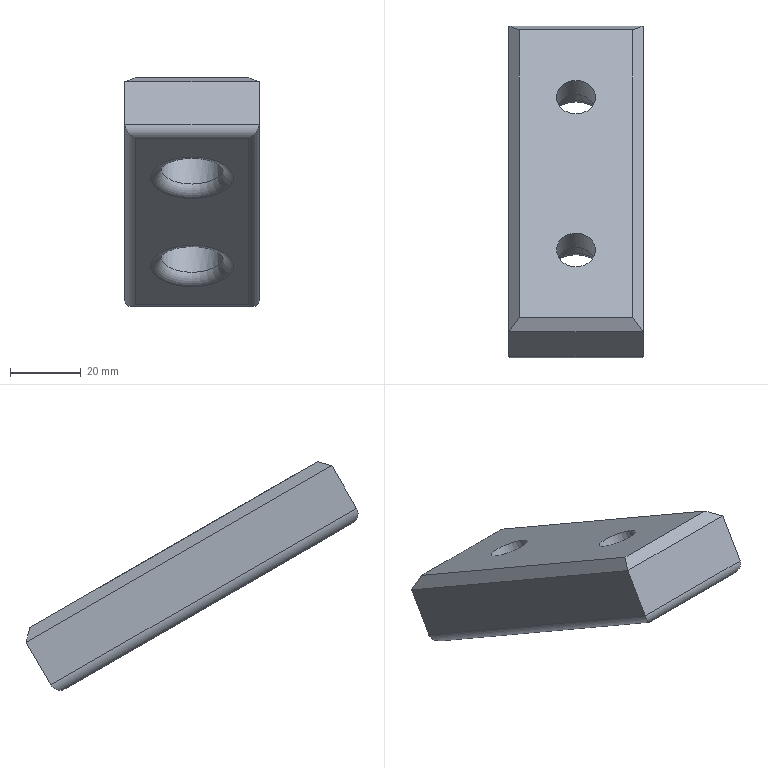Part | NX | features MAIN_BODY 2 | 1 solid | 22 faces | box 38 x 94.004 x 64.722 mm | volume 66749 mm3 | plane 12 | cylinder 8 | torus 2 | commonest cylinder face diameters 6 x4 11 x2 17.5 x2
STEP:
#1=CARTESIAN_POINT('',(222.,386.847,-246.44));
#2=VERTEX_POINT('',#1);
#3=CARTESIAN_POINT('',(222.,468.253,-293.44));
#4=VERTEX_POINT('',#3);
#5=CARTESIAN_POINT('',(222.,514.153,-319.94));
#6=DIRECTION('',(0.,-0.866,0.5));
#7=VECTOR('',#6,1000.);
#8=LINE('',#5,#7);
#9=EDGE_CURVE('',#2,#4,#8,.F.);
#10=ORIENTED_EDGE('',*,*,#9,.F.);
#11=CARTESIAN_POINT('',(190.,386.847,-246.44));
#12=VERTEX_POINT('',#11);
#13=CARTESIAN_POINT('',(225.,386.847,-246.44));
#14=DIRECTION('',(-1.,0.,0.));
#15=VECTOR('',#14,1000.);
#16=LINE('',#13,#15);
#17=EDGE_CURVE('',#12,#2,#16,.F.);
#18=ORIENTED_EDGE('',*,*,#17,.F.);
#19=CARTESIAN_POINT('',(190.,468.253,-293.44));
#20=VERTEX_POINT('',#19);
#21=CARTESIAN_POINT('',(190.,514.153,-319.94));
#22=DIRECTION('',(0.,0.866,-0.5));
#23=VECTOR('',#22,1000.);
#24=LINE('',#21,#23);
#25=EDGE_CURVE('',#20,#12,#24,.F.);
#26=ORIENTED_EDGE('',*,*,#25,.F.);
#27=CARTESIAN_POINT('',(225.,468.253,-293.44));
#28=DIRECTION('',(1.,0.,0.));
#29=VECTOR('',#28,1000.);
#30=LINE('',#27,#29);
#31=EDGE_CURVE('',#4,#20,#30,.F.);
#32=ORIENTED_EDGE('',*,*,#31,.F.);
#33=EDGE_LOOP('',(#10,#18,#26,#32));
#34=FACE_BOUND('',#33,.T.);
#35=CARTESIAN_POINT('',(206.,459.376,-288.315));
#36=VERTEX_POINT('',#35);
#37=CARTESIAN_POINT('',(206.,449.201,-282.44));
#38=DIRECTION('',(0.,0.5,0.866));
#39=DIRECTION('',(0.,0.866,-0.5));
#40=AXIS2_PLACEMENT_3D('',#37,#38,#39);
#41=CIRCLE('',#40,11.75);
#42=EDGE_CURVE('',#36,#36,#41,.F.);
#43=ORIENTED_EDGE('',*,*,#42,.F.);
#44=EDGE_LOOP('',(#43));
#45=FACE_BOUND('',#44,.T.);
#46=CARTESIAN_POINT('',(206.,416.075,-263.315));
#47=VERTEX_POINT('',#46);
#48=CARTESIAN_POINT('',(206.,405.899,-257.44));
#49=DIRECTION('',(0.,0.5,0.866));
#50=DIRECTION('',(0.,0.866,-0.5));
#51=AXIS2_PLACEMENT_3D('',#48,#49,#50);
#52=CIRCLE('',#51,11.75);
#53=EDGE_CURVE('',#47,#47,#52,.F.);
#54=ORIENTED_EDGE('',*,*,#53,.F.);
#55=EDGE_LOOP('',(#54));
#56=FACE_BOUND('',#55,.T.);
#57=CARTESIAN_POINT('',(225.,514.153,-319.94));
#58=DIRECTION('',(0.,-0.5,-0.866));
#59=DIRECTION('',(0.,0.866,-0.5));
#60=AXIS2_PLACEMENT_3D('',#57,#58,#59);
#61=PLANE('',#60);
#62=ADVANCED_FACE('',(#34,#45,#56),#61,.T.);
#63=CARTESIAN_POINT('',(200.5,459.201,-265.12));
#64=VERTEX_POINT('',#63);
#65=CARTESIAN_POINT('',(206.,459.201,-265.12));
#66=DIRECTION('',(0.,0.5,0.866));
#67=DIRECTION('',(-1.,0.,0.));
#68=AXIS2_PLACEMENT_3D('',#65,#66,#67);
#69=CIRCLE('',#68,5.5);
#70=EDGE_CURVE('',#64,#64,#69,.T.);
#71=ORIENTED_EDGE('',*,*,#70,.T.);
#72=EDGE_LOOP('',(#71));
#73=FACE_BOUND('',#72,.T.);
#74=CARTESIAN_POINT('',(206.,459.964,-274.798));
#75=VERTEX_POINT('',#74);
#76=CARTESIAN_POINT('',(206.,455.201,-272.048));
#77=DIRECTION('',(0.,0.5,0.866));
#78=DIRECTION('',(0.,0.866,-0.5));
#79=AXIS2_PLACEMENT_3D('',#76,#77,#78);
#80=CIRCLE('',#79,5.5);
#81=EDGE_CURVE('',#75,#75,#80,.T.);
#82=ORIENTED_EDGE('',*,*,#81,.F.);
#83=EDGE_LOOP('',(#82));
#84=FACE_BOUND('',#83,.T.);
#85=CARTESIAN_POINT('',(206.,449.201,-282.44));
#86=DIRECTION('',(0.,0.5,0.866));
#87=DIRECTION('',(0.,-0.866,0.5));
#88=AXIS2_PLACEMENT_3D('',#85,#86,#87);
#89=CYLINDRICAL_SURFACE('',#88,5.5);
#90=ADVANCED_FACE('',(#73,#84),#89,.F.);
#91=CARTESIAN_POINT('',(190.,396.847,-229.12));
#92=VERTEX_POINT('',#91);
#93=CARTESIAN_POINT('',(190.,478.253,-276.12));
#94=VERTEX_POINT('',#93);
#95=CARTESIAN_POINT('',(190.,524.153,-302.62));
#96=DIRECTION('',(0.,0.866,-0.5));
#97=VECTOR('',#96,1000.);
#98=LINE('',#95,#97);
#99=EDGE_CURVE('',#92,#94,#98,.T.);
#100=ORIENTED_EDGE('',*,*,#99,.F.);
#101=CARTESIAN_POINT('',(222.,396.847,-229.12));
#102=VERTEX_POINT('',#101);
#103=CARTESIAN_POINT('',(187.,396.847,-229.12));
#104=DIRECTION('',(-1.,0.,0.));
#105=VECTOR('',#104,1000.);
#106=LINE('',#103,#105);
#107=EDGE_CURVE('',#102,#92,#106,.T.);
#108=ORIENTED_EDGE('',*,*,#107,.F.);
#109=CARTESIAN_POINT('',(222.,478.253,-276.12));
#110=VERTEX_POINT('',#109);
#111=CARTESIAN_POINT('',(222.,394.249,-227.62));
#112=DIRECTION('',(0.,-0.866,0.5));
#113=VECTOR('',#112,1000.);
#114=LINE('',#111,#113);
#115=EDGE_CURVE('',#110,#102,#114,.T.);
#116=ORIENTED_EDGE('',*,*,#115,.F.);
#117=CARTESIAN_POINT('',(225.,478.253,-276.12));
#118=DIRECTION('',(1.,0.,0.));
#119=VECTOR('',#118,1000.);
#120=LINE('',#117,#119);
#121=EDGE_CURVE('',#94,#110,#120,.T.);
#122=ORIENTED_EDGE('',*,*,#121,.F.);
#123=EDGE_LOOP('',(#100,#108,#116,#122));
#124=FACE_BOUND('',#123,.T.);
#125=CARTESIAN_POINT('',(200.5,415.899,-240.12));
#126=VERTEX_POINT('',#125);
#127=CARTESIAN_POINT('',(206.,415.899,-240.12));
#128=DIRECTION('',(0.,-0.5,-0.866));
#129=DIRECTION('',(-1.,0.,0.));
#130=AXIS2_PLACEMENT_3D('',#127,#128,#129);
#131=CIRCLE('',#130,5.5);
#132=EDGE_CURVE('',#126,#126,#131,.T.);
#133=ORIENTED_EDGE('',*,*,#132,.T.);
#134=EDGE_LOOP('',(#133));
#135=FACE_BOUND('',#134,.T.);
#136=ORIENTED_EDGE('',*,*,#70,.F.);
#137=EDGE_LOOP('',(#136));
#138=FACE_BOUND('',#137,.T.);
#139=CARTESIAN_POINT('',(225.,524.153,-302.62));
#140=DIRECTION('',(0.,-0.5,-0.866));
#141=DIRECTION('',(0.,0.866,-0.5));
#142=AXIS2_PLACEMENT_3D('',#139,#140,#141);
#143=PLANE('',#142);
#144=ADVANCED_FACE('',(#124,#135,#138),#143,.F.);
#145=CARTESIAN_POINT('',(225.,385.749,-242.342));
#146=VERTEX_POINT('',#145);
#147=CARTESIAN_POINT('',(225.,392.749,-230.218));
#148=VERTEX_POINT('',#147);
#149=CARTESIAN_POINT('',(225.,384.249,-244.94));
#150=DIRECTION('',(0.,0.5,0.866));
#151=VECTOR('',#150,1000.);
#152=LINE('',#149,#151);
#153=EDGE_CURVE('',#146,#148,#152,.T.);
#154=ORIENTED_EDGE('',*,*,#153,.F.);
#155=CARTESIAN_POINT('',(225.,472.351,-292.342));
#156=VERTEX_POINT('',#155);
#157=CARTESIAN_POINT('',(225.,515.653,-317.342));
#158=DIRECTION('',(0.,-0.866,0.5));
#159=VECTOR('',#158,1000.);
#160=LINE('',#157,#159);
#161=EDGE_CURVE('',#156,#146,#160,.T.);
#162=ORIENTED_EDGE('',*,*,#161,.F.);
#163=CARTESIAN_POINT('',(225.,479.351,-280.218));
#164=VERTEX_POINT('',#163);
#165=CARTESIAN_POINT('',(225.,470.851,-294.94));
#166=DIRECTION('',(0.,0.5,0.866));
#167=VECTOR('',#166,1000.);
#168=LINE('',#165,#167);
#169=EDGE_CURVE('',#156,#164,#168,.T.);
#170=ORIENTED_EDGE('',*,*,#169,.T.);
#171=CARTESIAN_POINT('',(225.,522.653,-305.218));
#172=DIRECTION('',(0.,0.866,-0.5));
#173=VECTOR('',#172,1000.);
#174=LINE('',#171,#173);
#175=EDGE_CURVE('',#148,#164,#174,.T.);
#176=ORIENTED_EDGE('',*,*,#175,.F.);
#177=EDGE_LOOP('',(#154,#162,#170,#176));
#178=FACE_BOUND('',#177,.T.);
#179=CARTESIAN_POINT('',(225.,514.153,-319.94));
#180=DIRECTION('',(1.,0.,0.));
#181=DIRECTION('',(0.,0.866,-0.5));
#182=AXIS2_PLACEMENT_3D('',#179,#180,#181);
#183=PLANE('',#182);
#184=ADVANCED_FACE('',(#178),#183,.T.);
#185=CARTESIAN_POINT('',(187.,385.749,-242.342));
#186=VERTEX_POINT('',#185);
#187=CARTESIAN_POINT('',(187.,392.749,-230.218));
#188=VERTEX_POINT('',#187);
#189=CARTESIAN_POINT('',(187.,384.249,-244.94));
#190=DIRECTION('',(0.,0.5,0.866));
#191=VECTOR('',#190,1000.);
#192=LINE('',#189,#191);
#193=EDGE_CURVE('',#186,#188,#192,.T.);
#194=ORIENTED_EDGE('',*,*,#193,.F.);
#195=CARTESIAN_POINT('',(225.,385.749,-242.342));
#196=DIRECTION('',(-1.,0.,0.));
#197=VECTOR('',#196,1000.);
#198=LINE('',#195,#197);
#199=EDGE_CURVE('',#146,#186,#198,.T.);
#200=ORIENTED_EDGE('',*,*,#199,.F.);
#201=ORIENTED_EDGE('',*,*,#153,.T.);
#202=CARTESIAN_POINT('',(225.,392.749,-230.218));
#203=DIRECTION('',(1.,0.,0.));
#204=VECTOR('',#203,1000.);
#205=LINE('',#202,#204);
#206=EDGE_CURVE('',#188,#148,#205,.T.);
#207=ORIENTED_EDGE('',*,*,#206,.F.);
#208=EDGE_LOOP('',(#194,#200,#201,#207));
#209=FACE_BOUND('',#208,.T.);
#210=CARTESIAN_POINT('',(225.,384.249,-244.94));
#211=DIRECTION('',(0.,-0.866,0.5));
#212=DIRECTION('',(0.,-0.5,-0.866));
#213=AXIS2_PLACEMENT_3D('',#210,#211,#212);
#214=PLANE('',#213);
#215=ADVANCED_FACE('',(#209),#214,.T.);
#216=CARTESIAN_POINT('',(187.,472.351,-292.342));
#217=VERTEX_POINT('',#216);
#218=CARTESIAN_POINT('',(187.,479.351,-280.218));
#219=VERTEX_POINT('',#218);
#220=CARTESIAN_POINT('',(187.,470.851,-294.94));
#221=DIRECTION('',(0.,0.5,0.866));
#222=VECTOR('',#221,1000.);
#223=LINE('',#220,#222);
#224=EDGE_CURVE('',#217,#219,#223,.T.);
#225=ORIENTED_EDGE('',*,*,#224,.F.);
#226=CARTESIAN_POINT('',(187.,385.749,-242.342));
#227=DIRECTION('',(0.,0.866,-0.5));
#228=VECTOR('',#227,1000.);
#229=LINE('',#226,#228);
#230=EDGE_CURVE('',#186,#217,#229,.T.);
#231=ORIENTED_EDGE('',*,*,#230,.F.);
#232=ORIENTED_EDGE('',*,*,#193,.T.);
#233=CARTESIAN_POINT('',(187.,392.749,-230.218));
#234=DIRECTION('',(0.,-0.866,0.5));
#235=VECTOR('',#234,1000.);
#236=LINE('',#233,#235);
#237=EDGE_CURVE('',#219,#188,#236,.T.);
#238=ORIENTED_EDGE('',*,*,#237,.F.);
#239=EDGE_LOOP('',(#225,#231,#232,#238));
#240=FACE_BOUND('',#239,.T.);
#241=CARTESIAN_POINT('',(187.,384.249,-244.94));
#242=DIRECTION('',(-1.,0.,0.));
#243=DIRECTION('',(0.,-0.866,0.5));
#244=AXIS2_PLACEMENT_3D('',#241,#242,#243);
#245=PLANE('',#244);
#246=ADVANCED_FACE('',(#240),#245,.T.);
#247=ORIENTED_EDGE('',*,*,#169,.F.);
#248=CARTESIAN_POINT('',(187.,472.351,-292.342));
#249=DIRECTION('',(1.,0.,0.));
#250=VECTOR('',#249,1000.);
#251=LINE('',#248,#250);
#252=EDGE_CURVE('',#217,#156,#251,.T.);
#253=ORIENTED_EDGE('',*,*,#252,.F.);
#254=ORIENTED_EDGE('',*,*,#224,.T.);
#255=CARTESIAN_POINT('',(187.,479.351,-280.218));
#256=DIRECTION('',(-1.,0.,0.));
#257=VECTOR('',#256,1000.);
#258=LINE('',#255,#257);
#259=EDGE_CURVE('',#164,#219,#258,.T.);
#260=ORIENTED_EDGE('',*,*,#259,.F.);
#261=EDGE_LOOP('',(#247,#253,#254,#260));
#262=FACE_BOUND('',#261,.T.);
#263=CARTESIAN_POINT('',(187.,470.851,-294.94));
#264=DIRECTION('',(0.,0.866,-0.5));
#265=DIRECTION('',(-1.,0.,0.));
#266=AXIS2_PLACEMENT_3D('',#263,#264,#265);
#267=PLANE('',#266);
#268=ADVANCED_FACE('',(#262),#267,.T.);
#269=CARTESIAN_POINT('',(206.,407.136,-244.298));
#270=VERTEX_POINT('',#269);
#271=CARTESIAN_POINT('',(206.,411.899,-247.048));
#272=DIRECTION('',(0.,-0.5,-0.866));
#273=DIRECTION('',(0.,-0.866,0.5));
#274=AXIS2_PLACEMENT_3D('',#271,#272,#273);
#275=CIRCLE('',#274,5.5);
#276=EDGE_CURVE('',#270,#270,#275,.F.);
#277=ORIENTED_EDGE('',*,*,#276,.F.);
#278=EDGE_LOOP('',(#277));
#279=FACE_BOUND('',#278,.T.);
#280=ORIENTED_EDGE('',*,*,#132,.F.);
#281=EDGE_LOOP('',(#280));
#282=FACE_BOUND('',#281,.T.);
#283=CARTESIAN_POINT('',(206.,405.899,-257.44));
#284=DIRECTION('',(0.,0.5,0.866));
#285=DIRECTION('',(0.,-0.866,0.5));
#286=AXIS2_PLACEMENT_3D('',#283,#284,#285);
#287=CYLINDRICAL_SURFACE('',#286,5.5);
#288=ADVANCED_FACE('',(#279,#282),#287,.F.);
#289=CARTESIAN_POINT('',(206.,458.278,-284.217));
#290=VERTEX_POINT('',#289);
#291=CARTESIAN_POINT('',(206.,450.701,-279.842));
#292=DIRECTION('',(0.,0.5,0.866));
#293=DIRECTION('',(0.,0.866,-0.5));
#294=AXIS2_PLACEMENT_3D('',#291,#292,#293);
#295=CIRCLE('',#294,8.75);
#296=EDGE_CURVE('',#290,#290,#295,.T.);
#297=ORIENTED_EDGE('',*,*,#296,.F.);
#298=EDGE_LOOP('',(#297));
#299=FACE_BOUND('',#298,.T.);
#300=CARTESIAN_POINT('',(197.25,455.201,-272.048));
#301=VERTEX_POINT('',#300);
#302=CARTESIAN_POINT('',(206.,455.201,-272.048));
#303=DIRECTION('',(0.,0.5,0.866));
#304=DIRECTION('',(-1.,0.,0.));
#305=AXIS2_PLACEMENT_3D('',#302,#303,#304);
#306=CIRCLE('',#305,8.75);
#307=EDGE_CURVE('',#301,#301,#306,.T.);
#308=ORIENTED_EDGE('',*,*,#307,.T.);
#309=EDGE_LOOP('',(#308));
#310=FACE_BOUND('',#309,.T.);
#311=CARTESIAN_POINT('',(206.,444.201,-291.1));
#312=DIRECTION('',(0.,0.5,0.866));
#313=DIRECTION('',(0.,-0.866,0.5));
#314=AXIS2_PLACEMENT_3D('',#311,#312,#313);
#315=CYLINDRICAL_SURFACE('',#314,8.75);
#316=ADVANCED_FACE('',(#299,#310),#315,.F.);
#317=ORIENTED_EDGE('',*,*,#81,.T.);
#318=EDGE_LOOP('',(#317));
#319=FACE_BOUND('',#318,.T.);
#320=ORIENTED_EDGE('',*,*,#307,.F.);
#321=EDGE_LOOP('',(#320));
#322=FACE_BOUND('',#321,.T.);
#323=CARTESIAN_POINT('',(206.,455.201,-272.048));
#324=DIRECTION('',(0.,-0.5,-0.866));
#325=DIRECTION('',(0.,0.866,-0.5));
#326=AXIS2_PLACEMENT_3D('',#323,#324,#325);
#327=PLANE('',#326);
#328=ADVANCED_FACE('',(#319,#322),#327,.T.);
#329=CARTESIAN_POINT('',(197.25,411.899,-247.048));
#330=VERTEX_POINT('',#329);
#331=CARTESIAN_POINT('',(206.,411.899,-247.048));
#332=DIRECTION('',(0.,-0.5,-0.866));
#333=DIRECTION('',(-1.,0.,0.));
#334=AXIS2_PLACEMENT_3D('',#331,#332,#333);
#335=CIRCLE('',#334,8.75);
#336=EDGE_CURVE('',#330,#330,#335,.T.);
#337=ORIENTED_EDGE('',*,*,#336,.T.);
#338=EDGE_LOOP('',(#337));
#339=FACE_BOUND('',#338,.T.);
#340=ORIENTED_EDGE('',*,*,#276,.T.);
#341=EDGE_LOOP('',(#340));
#342=FACE_BOUND('',#341,.T.);
#343=CARTESIAN_POINT('',(206.,411.899,-247.048));
#344=DIRECTION('',(0.,0.5,0.866));
#345=DIRECTION('',(0.,-0.866,0.5));
#346=AXIS2_PLACEMENT_3D('',#343,#344,#345);
#347=PLANE('',#346);
#348=ADVANCED_FACE('',(#339,#342),#347,.F.);
#349=CARTESIAN_POINT('',(206.,414.977,-259.217));
#350=VERTEX_POINT('',#349);
#351=CARTESIAN_POINT('',(206.,407.399,-254.842));
#352=DIRECTION('',(0.,0.5,0.866));
#353=DIRECTION('',(0.,0.866,-0.5));
#354=AXIS2_PLACEMENT_3D('',#351,#352,#353);
#355=CIRCLE('',#354,8.75);
#356=EDGE_CURVE('',#350,#350,#355,.T.);
#357=ORIENTED_EDGE('',*,*,#356,.F.);
#358=EDGE_LOOP('',(#357));
#359=FACE_BOUND('',#358,.T.);
#360=ORIENTED_EDGE('',*,*,#336,.F.);
#361=EDGE_LOOP('',(#360));
#362=FACE_BOUND('',#361,.T.);
#363=CARTESIAN_POINT('',(206.,400.899,-266.1));
#364=DIRECTION('',(0.,0.5,0.866));
#365=DIRECTION('',(0.,-0.866,0.5));
#366=AXIS2_PLACEMENT_3D('',#363,#364,#365);
#367=CYLINDRICAL_SURFACE('',#366,8.75);
#368=ADVANCED_FACE('',(#359,#362),#367,.F.);
#369=CARTESIAN_POINT('',(222.,388.347,-243.842));
#370=DIRECTION('',(0.7071,0.6124,-0.3536));
#371=DIRECTION('',(-0.7071,0.6124,-0.3536));
#372=AXIS2_PLACEMENT_3D('',#369,#370,#371);
#373=ELLIPSE('',#372,4.243,3.);
#374=EDGE_CURVE('',#2,#146,#373,.F.);
#375=ORIENTED_EDGE('',*,*,#374,.T.);
#376=ORIENTED_EDGE('',*,*,#199,.T.);
#377=CARTESIAN_POINT('',(190.,388.347,-243.842));
#378=DIRECTION('',(0.7071,-0.6124,0.3536));
#379=DIRECTION('',(-0.7071,-0.6124,0.3536));
#380=AXIS2_PLACEMENT_3D('',#377,#378,#379);
#381=ELLIPSE('',#380,4.243,3.);
#382=EDGE_CURVE('',#186,#12,#381,.T.);
#383=ORIENTED_EDGE('',*,*,#382,.T.);
#384=ORIENTED_EDGE('',*,*,#17,.T.);
#385=EDGE_LOOP('',(#375,#376,#383,#384));
#386=FACE_BOUND('',#385,.T.);
#387=CARTESIAN_POINT('',(225.,388.347,-243.842));
#388=DIRECTION('',(-1.,0.,0.));
#389=DIRECTION('',(0.,-0.866,0.5));
#390=AXIS2_PLACEMENT_3D('',#387,#388,#389);
#391=CYLINDRICAL_SURFACE('',#390,3.);
#392=ADVANCED_FACE('',(#386),#391,.T.);
#393=ORIENTED_EDGE('',*,*,#382,.F.);
#394=ORIENTED_EDGE('',*,*,#230,.T.);
#395=CARTESIAN_POINT('',(190.,469.753,-290.842));
#396=DIRECTION('',(-0.7071,-0.6124,0.3536));
#397=DIRECTION('',(-0.7071,0.6124,-0.3536));
#398=AXIS2_PLACEMENT_3D('',#395,#396,#397);
#399=ELLIPSE('',#398,4.243,3.);
#400=EDGE_CURVE('',#217,#20,#399,.T.);
#401=ORIENTED_EDGE('',*,*,#400,.T.);
#402=ORIENTED_EDGE('',*,*,#25,.T.);
#403=EDGE_LOOP('',(#393,#394,#401,#402));
#404=FACE_BOUND('',#403,.T.);
#405=CARTESIAN_POINT('',(190.,385.749,-242.342));
#406=DIRECTION('',(0.,0.866,-0.5));
#407=DIRECTION('',(0.,0.5,0.866));
#408=AXIS2_PLACEMENT_3D('',#405,#406,#407);
#409=CYLINDRICAL_SURFACE('',#408,3.);
#410=ADVANCED_FACE('',(#404),#409,.T.);
#411=ORIENTED_EDGE('',*,*,#374,.F.);
#412=ORIENTED_EDGE('',*,*,#9,.T.);
#413=CARTESIAN_POINT('',(222.,469.753,-290.842));
#414=DIRECTION('',(-0.7071,0.6124,-0.3536));
#415=DIRECTION('',(-0.7071,-0.6124,0.3536));
#416=AXIS2_PLACEMENT_3D('',#413,#414,#415);
#417=ELLIPSE('',#416,4.243,3.);
#418=EDGE_CURVE('',#4,#156,#417,.F.);
#419=ORIENTED_EDGE('',*,*,#418,.T.);
#420=ORIENTED_EDGE('',*,*,#161,.T.);
#421=EDGE_LOOP('',(#411,#412,#419,#420));
#422=FACE_BOUND('',#421,.T.);
#423=CARTESIAN_POINT('',(222.,515.653,-317.342));
#424=DIRECTION('',(0.,-0.866,0.5));
#425=DIRECTION('',(1.,0.,0.));
#426=AXIS2_PLACEMENT_3D('',#423,#424,#425);
#427=CYLINDRICAL_SURFACE('',#426,3.);
#428=ADVANCED_FACE('',(#422),#427,.T.);
#429=ORIENTED_EDGE('',*,*,#400,.F.);
#430=ORIENTED_EDGE('',*,*,#252,.T.);
#431=ORIENTED_EDGE('',*,*,#418,.F.);
#432=ORIENTED_EDGE('',*,*,#31,.T.);
#433=EDGE_LOOP('',(#429,#430,#431,#432));
#434=FACE_BOUND('',#433,.T.);
#435=CARTESIAN_POINT('',(187.,469.753,-290.842));
#436=DIRECTION('',(1.,0.,0.));
#437=DIRECTION('',(0.,0.866,-0.5));
#438=AXIS2_PLACEMENT_3D('',#435,#436,#437);
#439=CYLINDRICAL_SURFACE('',#438,3.);
#440=ADVANCED_FACE('',(#434),#439,.T.);
#441=ORIENTED_EDGE('',*,*,#296,.T.);
#442=EDGE_LOOP('',(#441));
#443=FACE_BOUND('',#442,.T.);
#444=ORIENTED_EDGE('',*,*,#42,.T.);
#445=EDGE_LOOP('',(#444));
#446=FACE_BOUND('',#445,.T.);
#447=CARTESIAN_POINT('',(206.,450.701,-279.842));
#448=DIRECTION('',(0.,-0.5,-0.866));
#449=DIRECTION('',(0.,0.866,-0.5));
#450=AXIS2_PLACEMENT_3D('',#447,#448,#449);
#451=TOROIDAL_SURFACE('',#450,11.75,3.);
#452=ADVANCED_FACE('',(#443,#446),#451,.T.);
#453=ORIENTED_EDGE('',*,*,#53,.T.);
#454=EDGE_LOOP('',(#453));
#455=FACE_BOUND('',#454,.T.);
#456=ORIENTED_EDGE('',*,*,#356,.T.);
#457=EDGE_LOOP('',(#456));
#458=FACE_BOUND('',#457,.T.);
#459=CARTESIAN_POINT('',(206.,407.399,-254.842));
#460=DIRECTION('',(0.,-0.5,-0.866));
#461=DIRECTION('',(0.,0.866,-0.5));
#462=AXIS2_PLACEMENT_3D('',#459,#460,#461);
#463=TOROIDAL_SURFACE('',#462,11.75,3.);
#464=ADVANCED_FACE('',(#455,#458),#463,.T.);
#465=CARTESIAN_POINT('',(223.,395.481,-229.486));
#466=DIRECTION('',(0.5774,-0.7887,-0.2113));
#467=VECTOR('',#466,1000.);
#468=LINE('',#465,#467);
#469=EDGE_CURVE('',#148,#102,#468,.F.);
#470=ORIENTED_EDGE('',*,*,#469,.T.);
#471=ORIENTED_EDGE('',*,*,#107,.T.);
#472=CARTESIAN_POINT('',(239.,463.782,-211.184));
#473=DIRECTION('',(-0.5774,-0.7887,-0.2113));
#474=VECTOR('',#473,1000.);
#475=LINE('',#472,#474);
#476=EDGE_CURVE('',#92,#188,#475,.T.);
#477=ORIENTED_EDGE('',*,*,#476,.T.);
#478=ORIENTED_EDGE('',*,*,#206,.T.);
#479=EDGE_LOOP('',(#470,#471,#477,#478));
#480=FACE_BOUND('',#479,.T.);
#481=CARTESIAN_POINT('',(225.,396.847,-229.12));
#482=DIRECTION('',(0.,-0.2588,0.9659));
#483=DIRECTION('',(0.,-0.9659,-0.2588));
#484=AXIS2_PLACEMENT_3D('',#481,#482,#483);
#485=PLANE('',#484);
#486=ADVANCED_FACE('',(#480),#485,.T.);
#487=ORIENTED_EDGE('',*,*,#476,.F.);
#488=ORIENTED_EDGE('',*,*,#99,.T.);
#489=CARTESIAN_POINT('',(189.,478.619,-277.486));
#490=DIRECTION('',(0.5774,-0.2113,0.7887));
#491=VECTOR('',#490,1000.);
#492=LINE('',#489,#491);
#493=EDGE_CURVE('',#94,#219,#492,.F.);
#494=ORIENTED_EDGE('',*,*,#493,.T.);
#495=ORIENTED_EDGE('',*,*,#237,.T.);
#496=EDGE_LOOP('',(#487,#488,#494,#495));
#497=FACE_BOUND('',#496,.T.);
#498=CARTESIAN_POINT('',(190.,524.153,-302.62));
#499=DIRECTION('',(-0.7071,0.3536,0.6124));
#500=DIRECTION('',(0.7071,0.3536,0.6124));
#501=AXIS2_PLACEMENT_3D('',#498,#499,#500);
#502=PLANE('',#501);
#503=ADVANCED_FACE('',(#497),#502,.T.);
#504=ORIENTED_EDGE('',*,*,#469,.F.);
#505=ORIENTED_EDGE('',*,*,#175,.T.);
#506=CARTESIAN_POINT('',(223.,478.619,-277.486));
#507=DIRECTION('',(0.5774,0.2113,-0.7887));
#508=VECTOR('',#507,1000.);
#509=LINE('',#506,#508);
#510=EDGE_CURVE('',#164,#110,#509,.F.);
#511=ORIENTED_EDGE('',*,*,#510,.T.);
#512=ORIENTED_EDGE('',*,*,#115,.T.);
#513=EDGE_LOOP('',(#504,#505,#511,#512));
#514=FACE_BOUND('',#513,.T.);
#515=CARTESIAN_POINT('',(222.,524.153,-302.62));
#516=DIRECTION('',(0.7071,0.3536,0.6124));
#517=DIRECTION('',(0.7071,-0.3536,-0.6124));
#518=AXIS2_PLACEMENT_3D('',#515,#516,#517);
#519=PLANE('',#518);
#520=ADVANCED_FACE('',(#514),#519,.T.);
#521=ORIENTED_EDGE('',*,*,#493,.F.);
#522=ORIENTED_EDGE('',*,*,#121,.T.);
#523=ORIENTED_EDGE('',*,*,#510,.F.);
#524=ORIENTED_EDGE('',*,*,#259,.T.);
#525=EDGE_LOOP('',(#521,#522,#523,#524));
#526=FACE_BOUND('',#525,.T.);
#527=CARTESIAN_POINT('',(225.,478.253,-276.12));
#528=DIRECTION('',(0.,0.9659,0.2588));
#529=DIRECTION('',(0.,-0.2588,0.9659));
#530=AXIS2_PLACEMENT_3D('',#527,#528,#529);
#531=PLANE('',#530);
#532=ADVANCED_FACE('',(#526),#531,.T.);
#533=CLOSED_SHELL('',(#62,#90,#144,#184,#215,#246,#268,#288,#316,#328,#348,#368,#392,#410,#428,#440,#452,#464,#486,#503,#520,#532));
#534=MANIFOLD_SOLID_BREP('',#533);
#535=(LENGTH_UNIT()NAMED_UNIT(*)SI_UNIT(.MILLI.,.METRE.));
#536=UNCERTAINTY_MEASURE_WITH_UNIT(LENGTH_MEASURE(0.00001),#535,'','');
#537=(NAMED_UNIT(*)PLANE_ANGLE_UNIT()SI_UNIT($,.RADIAN.));
#538=(NAMED_UNIT(*)SI_UNIT($,.STERADIAN.)SOLID_ANGLE_UNIT());
#539=(GEOMETRIC_REPRESENTATION_CONTEXT(3)GLOBAL_UNCERTAINTY_ASSIGNED_CONTEXT((#536))GLOBAL_UNIT_ASSIGNED_CONTEXT((#535,#537,#538))REPRESENTATION_CONTEXT('',''));
#540=ADVANCED_BREP_SHAPE_REPRESENTATION('',(#534),#539);